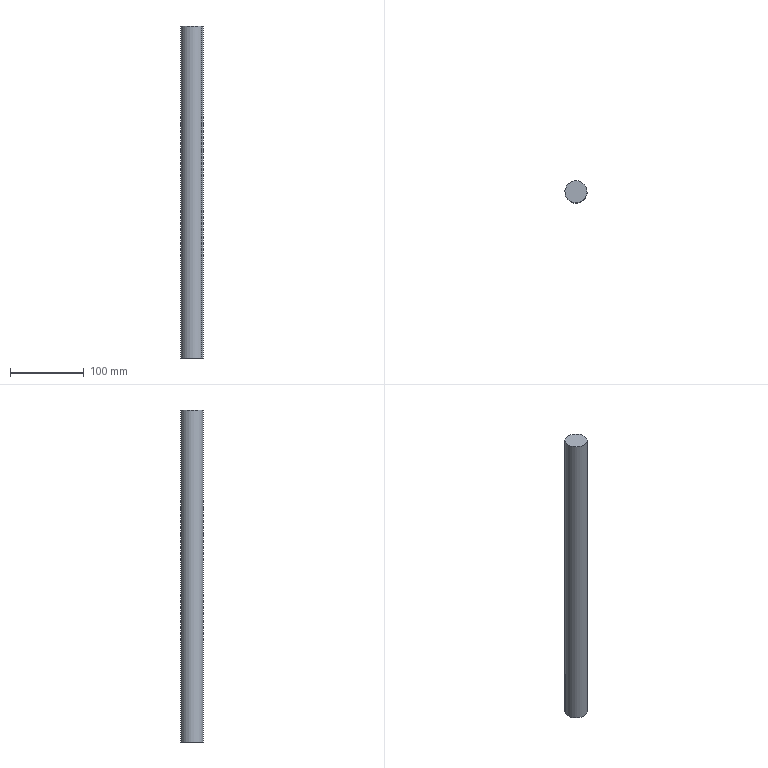Part | STEP file | Boss-Extrude 1-2 | 1 solid | 4 faces | box 30 x 30 x 450 mm | volume 318086 mm3 | cylinder 2 | plane 2 | commonest cylinder face diameters 30 x2
STEP:
#1=CARTESIAN_POINT('',(-1375.973,1726.387,3033.5));
#2=VERTEX_POINT('',#1);
#3=CARTESIAN_POINT('',(-1401.503,1742.142,3033.5));
#4=VERTEX_POINT('',#3);
#5=CARTESIAN_POINT('',(-1388.738,1734.264,3033.5));
#6=DIRECTION('',(0.,0.,1.));
#7=DIRECTION('',(0.851,-0.5251,0.));
#8=AXIS2_PLACEMENT_3D('',#5,#6,#7);
#9=CIRCLE('',#8,15.);
#10=EDGE_CURVE('',#2,#4,#9,.T.);
#11=ORIENTED_EDGE('',*,*,#10,.F.);
#12=CARTESIAN_POINT('',(-1375.973,1726.387,2583.5));
#13=VERTEX_POINT('',#12);
#14=CARTESIAN_POINT('',(-1375.973,1726.387,3033.5));
#15=DIRECTION('',(0.,0.,-1.));
#16=VECTOR('',#15,1000.);
#17=LINE('',#14,#16);
#18=EDGE_CURVE('',#2,#13,#17,.T.);
#19=ORIENTED_EDGE('',*,*,#18,.T.);
#20=CARTESIAN_POINT('',(-1401.503,1742.142,2583.5));
#21=VERTEX_POINT('',#20);
#22=CARTESIAN_POINT('',(-1388.738,1734.264,2583.5));
#23=DIRECTION('',(0.,0.,1.));
#24=DIRECTION('',(0.851,-0.5251,0.));
#25=AXIS2_PLACEMENT_3D('',#22,#23,#24);
#26=CIRCLE('',#25,15.);
#27=EDGE_CURVE('',#13,#21,#26,.T.);
#28=ORIENTED_EDGE('',*,*,#27,.T.);
#29=CARTESIAN_POINT('',(-1401.503,1742.142,3033.5));
#30=DIRECTION('',(0.,0.,-1.));
#31=VECTOR('',#30,1000.);
#32=LINE('',#29,#31);
#33=EDGE_CURVE('',#4,#21,#32,.T.);
#34=ORIENTED_EDGE('',*,*,#33,.F.);
#35=EDGE_LOOP('',(#11,#19,#28,#34));
#36=FACE_OUTER_BOUND('',#35,.T.);
#37=CARTESIAN_POINT('',(-1388.738,1734.264,3033.5));
#38=DIRECTION('',(0.,0.,-1.));
#39=DIRECTION('',(0.851,-0.5251,0.));
#40=AXIS2_PLACEMENT_3D('',#37,#38,#39);
#41=CYLINDRICAL_SURFACE('',#40,15.);
#42=ADVANCED_FACE('',(#36),#41,.T.);
#43=ORIENTED_EDGE('',*,*,#18,.F.);
#44=CARTESIAN_POINT('',(-1388.738,1734.264,3033.5));
#45=DIRECTION('',(0.,0.,1.));
#46=DIRECTION('',(0.851,-0.5251,0.));
#47=AXIS2_PLACEMENT_3D('',#44,#45,#46);
#48=CIRCLE('',#47,15.);
#49=EDGE_CURVE('',#4,#2,#48,.T.);
#50=ORIENTED_EDGE('',*,*,#49,.F.);
#51=ORIENTED_EDGE('',*,*,#33,.T.);
#52=CARTESIAN_POINT('',(-1388.738,1734.264,2583.5));
#53=DIRECTION('',(0.,0.,1.));
#54=DIRECTION('',(0.851,-0.5251,0.));
#55=AXIS2_PLACEMENT_3D('',#52,#53,#54);
#56=CIRCLE('',#55,15.);
#57=EDGE_CURVE('',#21,#13,#56,.T.);
#58=ORIENTED_EDGE('',*,*,#57,.T.);
#59=EDGE_LOOP('',(#43,#50,#51,#58));
#60=FACE_OUTER_BOUND('',#59,.T.);
#61=CARTESIAN_POINT('',(-1388.738,1734.264,3033.5));
#62=DIRECTION('',(0.,0.,-1.));
#63=DIRECTION('',(0.851,-0.5251,0.));
#64=AXIS2_PLACEMENT_3D('',#61,#62,#63);
#65=CYLINDRICAL_SURFACE('',#64,15.);
#66=ADVANCED_FACE('',(#60),#65,.T.);
#67=ORIENTED_EDGE('',*,*,#49,.T.);
#68=ORIENTED_EDGE('',*,*,#10,.T.);
#69=EDGE_LOOP('',(#67,#68));
#70=FACE_OUTER_BOUND('',#69,.T.);
#71=CARTESIAN_POINT('',(-1388.738,1734.264,3033.5));
#72=DIRECTION('',(0.,0.,1.));
#73=DIRECTION('',(-0.851,0.5251,0.));
#74=AXIS2_PLACEMENT_3D('',#71,#72,#73);
#75=PLANE('',#74);
#76=ADVANCED_FACE('',(#70),#75,.T.);
#77=ORIENTED_EDGE('',*,*,#57,.F.);
#78=ORIENTED_EDGE('',*,*,#27,.F.);
#79=EDGE_LOOP('',(#77,#78));
#80=FACE_OUTER_BOUND('',#79,.T.);
#81=CARTESIAN_POINT('',(-1388.738,1734.264,2583.5));
#82=DIRECTION('',(0.,0.,1.));
#83=DIRECTION('',(-0.851,0.5251,0.));
#84=AXIS2_PLACEMENT_3D('',#81,#82,#83);
#85=PLANE('',#84);
#86=ADVANCED_FACE('',(#80),#85,.F.);
#87=CLOSED_SHELL('',(#42,#66,#76,#86));
#88=MANIFOLD_SOLID_BREP('',#87);
#89=CARTESIAN_POINT('',(0.,0.,0.));
#90=DIRECTION('',(0.,0.,1.));
#91=DIRECTION('',(1.,0.,0.));
#92=AXIS2_PLACEMENT_3D('',#89,#90,#91);
#93=(LENGTH_UNIT()NAMED_UNIT(*)SI_UNIT(.MILLI.,.METRE.));
#94=UNCERTAINTY_MEASURE_WITH_UNIT(LENGTH_MEASURE(0.00001),#93,'','');
#95=(NAMED_UNIT(*)PLANE_ANGLE_UNIT()SI_UNIT($,.RADIAN.));
#96=(NAMED_UNIT(*)SI_UNIT($,.STERADIAN.)SOLID_ANGLE_UNIT());
#97=(GEOMETRIC_REPRESENTATION_CONTEXT(3)GLOBAL_UNCERTAINTY_ASSIGNED_CONTEXT((#94))GLOBAL_UNIT_ASSIGNED_CONTEXT((#93,#95,#96))REPRESENTATION_CONTEXT('',''));
#98=ADVANCED_BREP_SHAPE_REPRESENTATION('',(#88,#92),#97);